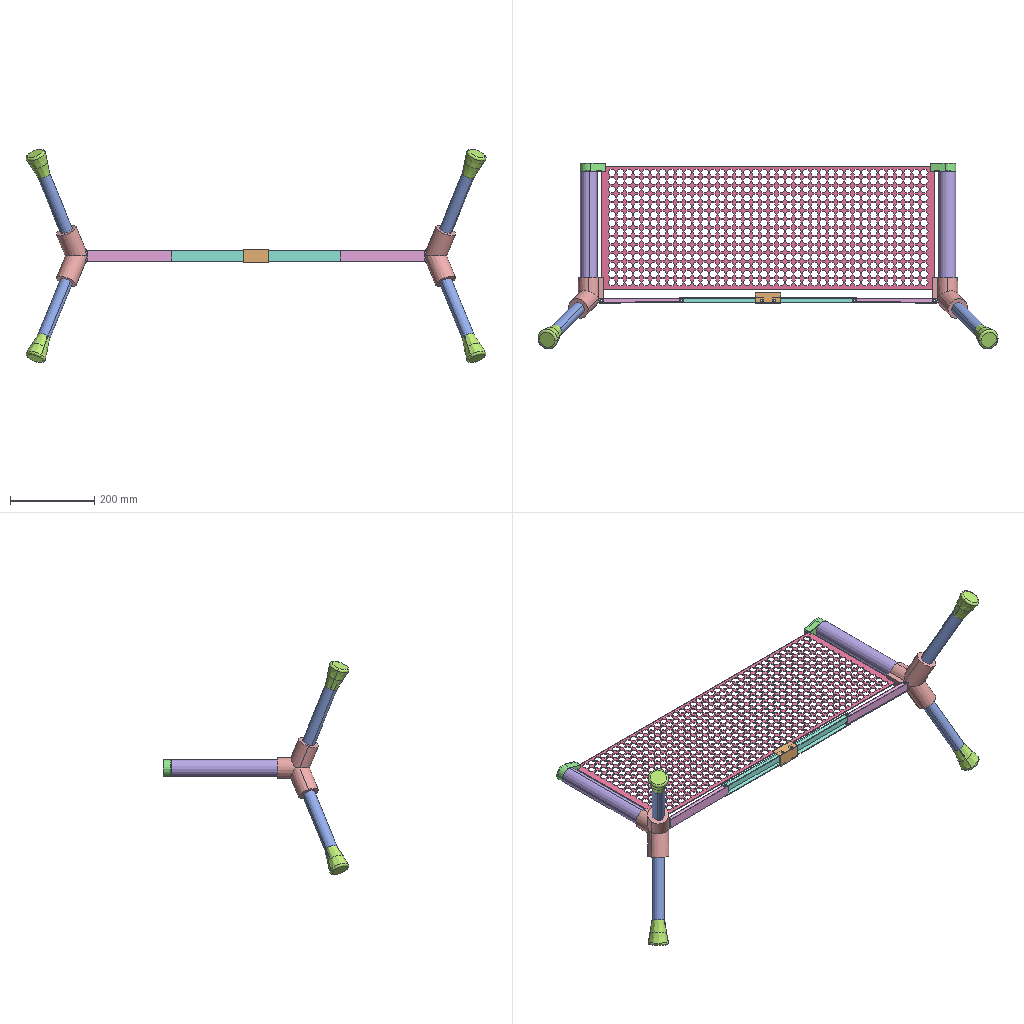Assembly | SolidWorks | 9 different items | 20 placed | box 1090 x 440 x 505 mm
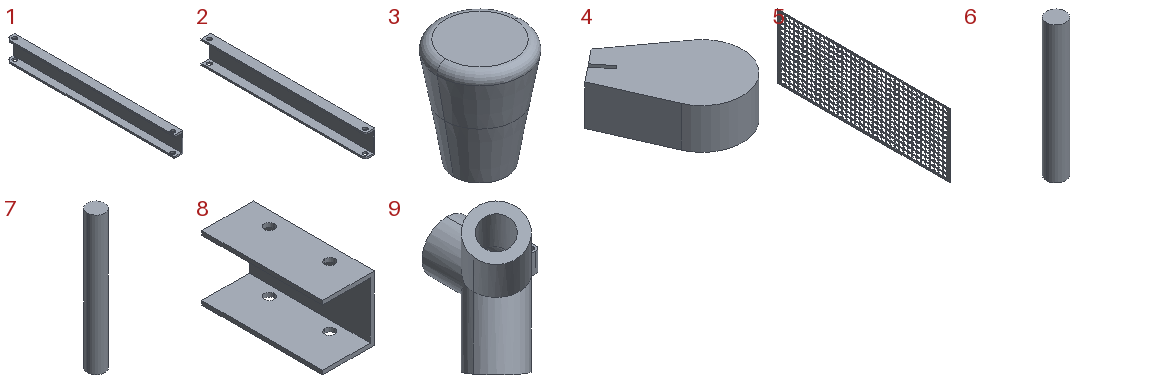Parts list (item | quantity | size | volume | features):
1 | x2 | 10 x 200 x 24 mm | 15821 mm3 | features Cut 2, Extrusion 1, Fillet 1
2 | x2 | 12 x 200 x 28 mm | 19021 mm3 | features Cut 2, Extrusion 1, Fillet 1
3 | x4 | 48.662 x 48.662 x 60 mm | 55216 mm3 | features Extrusion 1, Fillet 1, ICE 1, RevCut 1
4 | x2 | 52.852 x 57.443 x 20 mm | 11809 mm3 | features Cut 2, Extrusion 1, Shell 1
5 | x1 | - | 218859 mm3 | features ICE 2, Cut 1, Extrusion 1, LPattern 1
6 | x2 | 40 x 40 x 280 mm | 351858 mm3 | features Extrusion 1
7 | x4 | 30 x 30 x 240 mm | 169646 mm3 | features Extrusion 1
8 | x1 | 25.474 x 60 x 32 mm | 9317 mm3 | features Cut 1, Extrusion 1, MirrorPattern 1
9 | x2 | 83.134 x 98.134 x 146.244 mm | 202808 mm3 | features Cut 5, ICE 4, 3DProfileFeature 2, Fillet 1, RefAxis 1, Sweep 1
Mates (type | each side: item.copy, entity, surface, feature):
Concentric | 9.1 face cylinder Cut-Extrude1 | 7.1 face cylinder Boss-Extrude1
Coincident | 9.1 face plane Cut-Extrude1 | 7.1 face plane Boss-Extrude1
Coincident | 7.1 face plane Boss-Extrude1 | 3.1 face plane Boss-Extrude1
Concentric | 7.1 edge | 3.1 edge
Coincident | 7.2 face plane Boss-Extrude1 | 3.2 face plane Boss-Extrude1
Concentric | 7.2 edge | 3.2 edge
Concentric | 9.1 face cylinder Cut-Extrude2 | 7.2 face cylinder Boss-Extrude1
Coincident | 9.1 face plane Cut-Extrude2 | 7.2 face plane Boss-Extrude1
Concentric | 9.1 face cylinder Cut-Extrude4 | 1.1 face cylinder Cut-Extrude1
Coincident | 9.1 face plane Boss-Extrude5 | 1.1 face plane Boss-Extrude1
LimitPlanarAngleDim | 1.1 face plane Boss-Extrude1 | 9.1 face plane Boss-Extrude5
Concentric | 1.1 face cylinder Cut-Extrude2 | 2.1 face cylinder Cut-Extrude2
Coincident | 1.1 edge | 2.1 edge
LimitPlanarAngleDim | 2.1 face plane Boss-Extrude1 | 1.1 face plane Boss-Extrude1
Concentric | 2.1 face cylinder Cut-Extrude1 | 8.1 face cylinder Mirror1
Coincident | 2.1 edge | 8.1 edge
LimitPlanarAngleDim | 8.1 face plane Boss-Extrude1 | 2.1 face plane Boss-Extrude1
Concentric | 9.1 face cylinder Cut-Extrude3 | 6.1 face cylinder Boss-Extrude1
DistanceDim | 6.1 face plane Boss-Extrude1 | 9.1 face plane Boss-Extrude1
Concentric | 9.2 face cylinder Cut-Extrude3 | 6.2 face cylinder Boss-Extrude1
DistanceDim | 6.2 face plane Boss-Extrude1 | 9.2 face plane Boss-Extrude1
Coincident | 9.1 face plane Boss-Extrude1 | 9.2 face plane Boss-Extrude1
Concentric | 6.1 face cylinder Boss-Extrude1 | 4.1 face cylinder Boss-Extrude1
Coincident | 6.1 edge | 4.1 face plane Boss-Extrude1
Parallel | 9.1 edge | 4.1 edge
Concentric | 6.2 face cylinder Boss-Extrude1 | 4.2 face cylinder Boss-Extrude1
Coincident | 6.2 face plane Boss-Extrude1 | 4.2 face plane Boss-Extrude1
Parallel | 9.2 edge | 4.2 edge
Width | 4.1 face plane Cut-Extrude1 | 4.1 face plane Cut-Extrude1 | 5.1 face plane Boss-Extrude1 | 5.1 face plane Boss-Extrude1
Width | 4.1 face plane Cut-Extrude2 | 4.2 face plane Cut-Extrude2 | 5.1 face plane Boss-Extrude2 | 5.1 face plane Boss-Extrude3